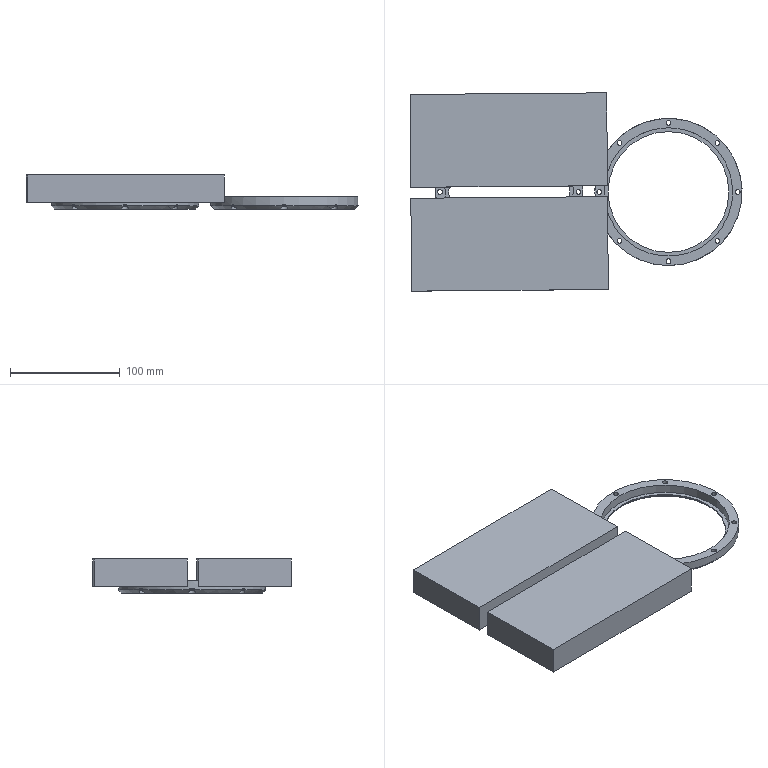Part | 4 solids | 80 faces | box 302.234 x 180.468 x 31 mm | volume 764664 mm3 | cylinder 40 | plane 36 | cone 4 | commonest cylinder face diameters 4.3 x16 7 x16 134 x4 110 x2 117 x2